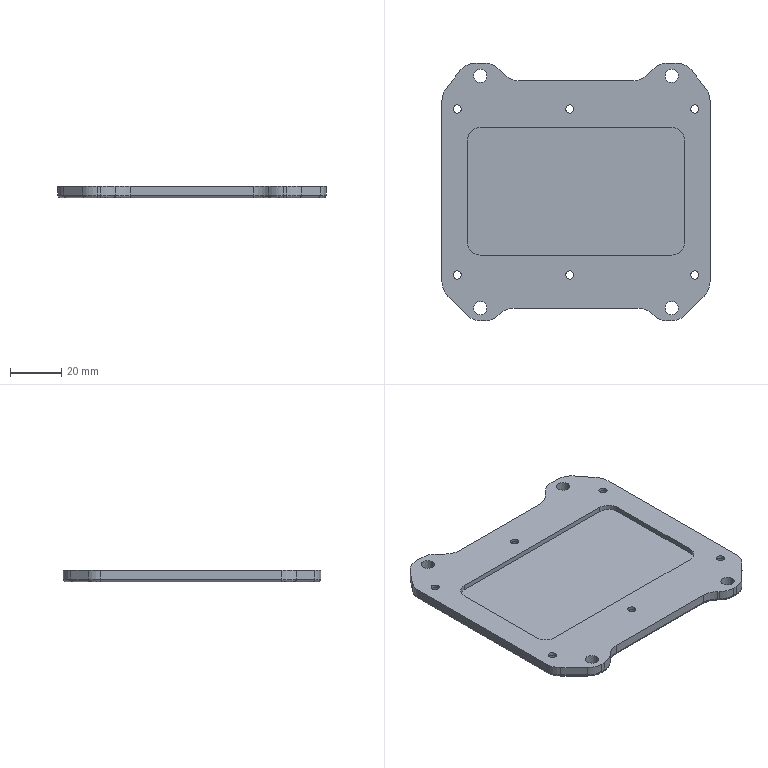NC program | NX | posted with a generic post | part box 105 x 101 x 4.5 mm
Lines 736 to 1574 of 30641:
(PLANAR_MILL_1 , TOOL : D4-12-D4-50-3T-FINISH)
N1452 T04 M6
N1454 G53
N1456 G17 G0 G90 X-47.229 Y-31.877 S4500 M3
N1458 G43 Z20. H4
N1460 Z0.5
N1462 G94 G1 X-47.45 Y-32.259 Z0.485 F500.
N1464 Y-32.741 Z0.468
N1466 X-47.183 Y-33.202 Z0.449
N1468 X-46.767 Y-33.443 Z0.432
N1470 X-46.251 Y-33.448 Z0.414
N1472 X-45.804 Y-33.19 Z0.396
N1474 X-45.55 Y-32.741 Z0.378
N1476 Y-32.259 Z0.362
N1478 X-45.804 Y-31.81 Z0.343
N1480 X-46.251 Y-31.552 Z0.325
N1482 X-46.767 Y-31.557 Z0.307
N1484 X-47.183 Y-31.798 Z0.291
N1486 X-47.45 Y-32.259 Z0.272
N1488 Y-32.741 Z0.255
N1490 X-47.183 Y-33.202 Z0.237
N1492 X-46.767 Y-33.443 Z0.22
N1494 X-46.251 Y-33.448 Z0.202
N1496 X-45.804 Y-33.19 Z0.184
N1498 X-45.55 Y-32.741 Z0.166
N1500 Y-32.259 Z0.149
N1502 X-45.804 Y-31.81 Z0.131
N1504 X-46.251 Y-31.552 Z0.113
N1506 X-46.767 Y-31.557 Z0.095
N1508 X-47.183 Y-31.798 Z0.078
N1510 X-47.45 Y-32.259 Z0.059
N1512 Y-32.741 Z0.043
N1514 X-47.183 Y-33.202 Z0.024
N1516 X-46.767 Y-33.443 Z0.007
N1518 X-46.251 Y-33.448 Z-0.011
N1520 X-45.804 Y-33.19 Z-0.029
N1522 X-45.55 Y-32.741 Z-0.047
N1524 Y-32.259 Z-0.064
N1526 X-45.804 Y-31.81 Z-0.082
N1528 X-46.251 Y-31.552 Z-0.1
N1530 X-46.767 Y-31.557 Z-0.118
N1532 X-47.183 Y-31.798 Z-0.134
N1534 X-47.45 Y-32.259 Z-0.153
N1536 Y-32.741 Z-0.17
N1538 X-47.183 Y-33.202 Z-0.189
N1540 X-46.767 Y-33.443 Z-0.205
N1542 X-46.251 Y-33.448 Z-0.223
N1544 X-45.804 Y-33.19 Z-0.241
N1546 X-45.55 Y-32.741 Z-0.259
N1548 Y-32.259 Z-0.276
N1550 X-45.804 Y-31.81 Z-0.294
N1552 X-46.251 Y-31.552 Z-0.312
N1554 X-46.767 Y-31.557 Z-0.33
N1556 X-47.183 Y-31.798 Z-0.347
N1558 X-47.45 Y-32.259 Z-0.366
N1560 Y-32.741 Z-0.382
N1562 X-47.183 Y-33.202 Z-0.401
N1564 X-46.767 Y-33.443 Z-0.418
N1566 X-46.251 Y-33.448 Z-0.436
N1568 X-45.804 Y-33.19 Z-0.454
N1570 X-45.55 Y-32.741 Z-0.472
N1572 Y-32.259 Z-0.489
N1574 X-45.804 Y-31.81 Z-0.507
N1576 X-46.251 Y-31.552 Z-0.525
N1578 X-46.767 Y-31.557 Z-0.543
N1580 X-47.183 Y-31.798 Z-0.56
N1582 X-47.45 Y-32.259 Z-0.578
N1584 Y-32.741 Z-0.595
N1586 X-47.183 Y-33.202 Z-0.614
N1588 X-46.767 Y-33.443 Z-0.63
N1590 X-46.251 Y-33.448 Z-0.648
N1592 X-45.804 Y-33.19 Z-0.667
N1594 X-45.55 Y-32.741 Z-0.685
N1596 Y-32.259 Z-0.701
N1598 X-45.804 Y-31.81 Z-0.719
N1600 X-46.251 Y-31.552 Z-0.737
N1602 X-46.767 Y-31.557 Z-0.755
N1604 X-47.183 Y-31.798 Z-0.772
N1606 X-47.45 Y-32.259 Z-0.791
N1608 Y-32.741 Z-0.808
N1610 X-47.183 Y-33.202 Z-0.826
N1612 X-46.767 Y-33.443 Z-0.843
N1614 X-46.251 Y-33.448 Z-0.861
N1616 X-45.804 Y-33.19 Z-0.879
N1618 X-45.55 Y-32.741 Z-0.897
N1620 Y-32.259 Z-0.914
N1622 X-45.804 Y-31.81 Z-0.932
N1624 X-46.251 Y-31.552 Z-0.95
N1626 X-46.767 Y-31.557 Z-0.968
N1628 X-47.183 Y-31.798 Z-0.985
N1630 X-47.45 Y-32.259 Z-1.003
N1632 Y-32.741 Z-1.02
N1634 X-47.183 Y-33.202 Z-1.039
N1636 X-46.767 Y-33.443 Z-1.056
N1638 X-46.251 Y-33.448 Z-1.074
N1640 X-45.804 Y-33.19 Z-1.092
N1642 X-45.55 Y-32.741 Z-1.11
N1644 Y-32.259 Z-1.126
N1646 X-45.804 Y-31.81 Z-1.144
N1648 X-46.251 Y-31.552 Z-1.162
N1650 X-46.767 Y-31.557 Z-1.181
N1652 X-47.183 Y-31.798 Z-1.197
N1654 X-47.45 Y-32.259 Z-1.216
N1656 Y-32.741 Z-1.233
N1658 X-47.183 Y-33.202 Z-1.251
N1660 X-46.767 Y-33.443 Z-1.268
N1662 X-46.251 Y-33.448 Z-1.286
N1664 X-45.804 Y-33.19 Z-1.304
N1666 X-45.55 Y-32.741 Z-1.322
N1668 Y-32.259 Z-1.339
N1670 X-45.804 Y-31.81 Z-1.357
N1672 X-46.251 Y-31.552 Z-1.375
N1674 X-46.767 Y-31.557 Z-1.393
N1676 X-47.183 Y-31.798 Z-1.41
N1678 X-47.45 Y-32.259 Z-1.429
N1680 Y-32.741 Z-1.445
N1682 X-47.183 Y-33.202 Z-1.464
N1684 X-46.767 Y-33.443 Z-1.481
N1686 X-46.251 Y-33.448 Z-1.499
N1688 X-45.804 Y-33.19 Z-1.517
N1690 X-45.55 Y-32.741 Z-1.535
N1692 Y-32.259 Z-1.552
N1694 X-45.804 Y-31.81 Z-1.57
N1696 X-46.251 Y-31.552 Z-1.588
N1698 X-46.767 Y-31.557 Z-1.606
N1700 X-47.183 Y-31.798 Z-1.622
N1702 X-47.45 Y-32.259 Z-1.641
N1704 Y-32.741 Z-1.658
N1706 X-47.183 Y-33.202 Z-1.676
N1708 X-46.767 Y-33.443 Z-1.693
N1710 X-46.251 Y-33.448 Z-1.711
N1712 X-45.804 Y-33.19 Z-1.729
N1714 X-45.55 Y-32.741 Z-1.747
N1716 Y-32.259 Z-1.764
N1718 X-45.804 Y-31.81 Z-1.782
N1720 X-46.251 Y-31.552 Z-1.8
N1722 X-46.767 Y-31.557 Z-1.818
N1724 X-47.183 Y-31.798 Z-1.835
N1726 X-47.45 Y-32.259 Z-1.854
N1728 Y-32.741 Z-1.87
N1730 X-47.183 Y-33.202 Z-1.889
N1732 X-46.767 Y-33.443 Z-1.906
N1734 X-46.251 Y-33.448 Z-1.924
N1736 X-45.804 Y-33.19 Z-1.942
N1738 X-45.55 Y-32.741 Z-1.96
N1740 Y-32.259 Z-1.977
N1742 X-45.804 Y-31.81 Z-1.995
N1744 X-46.251 Y-31.552 Z-2.013
N1746 X-46.767 Y-31.557 Z-2.031
N1748 X-47.183 Y-31.798 Z-2.048
N1750 X-47.45 Y-32.259 Z-2.066
N1752 Y-32.741 Z-2.083
N1754 X-47.183 Y-33.202 Z-2.102
N1756 X-46.767 Y-33.443 Z-2.118
N1758 X-46.251 Y-33.448 Z-2.136
N1760 X-45.804 Y-33.19 Z-2.154
N1762 X-45.55 Y-32.741 Z-2.172
N1764 Y-32.259 Z-2.189
N1766 X-45.804 Y-31.81 Z-2.207
N1768 X-46.251 Y-31.552 Z-2.225
N1770 X-46.767 Y-31.557 Z-2.243
N1772 X-47.183 Y-31.798 Z-2.26
N1774 X-47.45 Y-32.259 Z-2.279
N1776 Y-32.741 Z-2.296
N1778 X-47.183 Y-33.202 Z-2.314
N1780 X-46.767 Y-33.443 Z-2.331
N1782 X-46.251 Y-33.448 Z-2.349
N1784 X-45.804 Y-33.19 Z-2.367
N1786 X-45.55 Y-32.741 Z-2.385
N1788 Y-32.259 Z-2.402
N1790 X-45.804 Y-31.81 Z-2.42
N1792 X-46.251 Y-31.552 Z-2.438
N1794 X-46.767 Y-31.557 Z-2.456
N1796 X-47.183 Y-31.798 Z-2.473
N1798 X-47.45 Y-32.259 Z-2.491
N1800 Y-32.741 Z-2.508
N1802 X-47.183 Y-33.202 Z-2.527
N1804 X-46.767 Y-33.443 Z-2.544
N1806 X-46.251 Y-33.448 Z-2.562
N1808 X-45.804 Y-33.19 Z-2.58
N1810 X-45.55 Y-32.741 Z-2.598
N1812 Y-32.259 Z-2.614
N1814 X-45.804 Y-31.81 Z-2.632
N1816 X-46.251 Y-31.552 Z-2.65
N1818 X-46.767 Y-31.557 Z-2.668
N1820 X-47.183 Y-31.798 Z-2.685
N1822 X-47.45 Y-32.259 Z-2.704
N1824 Y-32.741 Z-2.721
N1826 X-47.183 Y-33.202 Z-2.739
N1828 X-46.767 Y-33.443 Z-2.756
N1830 X-46.251 Y-33.448 Z-2.774
N1832 X-45.804 Y-33.19 Z-2.792
N1834 X-45.55 Y-32.741 Z-2.81
N1836 Y-32.259 Z-2.827
N1838 X-45.804 Y-31.81 Z-2.845
N1840 X-46.251 Y-31.552 Z-2.863
N1842 X-46.767 Y-31.557 Z-2.881
N1844 X-47.183 Y-31.798 Z-2.898
N1846 X-47.45 Y-32.259 Z-2.916
N1848 Y-32.741 Z-2.933
N1850 X-47.183 Y-33.202 Z-2.952
N1852 X-46.767 Y-33.443 Z-2.969
N1854 X-46.251 Y-33.448 Z-2.987
N1856 X-45.804 Y-33.19 Z-3.005
N1858 X-45.55 Y-32.741 Z-3.023
N1860 Y-32.259 Z-3.04
N1862 X-45.804 Y-31.81 Z-3.058
N1864 X-46.251 Y-31.552 Z-3.076
N1866 X-46.767 Y-31.557 Z-3.094
N1868 X-47.183 Y-31.798 Z-3.11
N1870 X-47.45 Y-32.259 Z-3.129
N1872 Y-32.741 Z-3.146
N1874 X-47.183 Y-33.202 Z-3.164
N1876 X-46.767 Y-33.443 Z-3.181
N1878 X-46.251 Y-33.448 Z-3.199
N1880 X-45.804 Y-33.19 Z-3.217
N1882 X-45.55 Y-32.741 Z-3.235
N1884 Y-32.259 Z-3.252
N1886 X-45.804 Y-31.81 Z-3.27
N1888 X-46.251 Y-31.552 Z-3.288
N1890 X-46.767 Y-31.557 Z-3.306
N1892 X-47.183 Y-31.798 Z-3.323
N1894 X-47.45 Y-32.259 Z-3.342
N1896 Y-32.5 Z-3.35
N1898 G3 X-46.5 Y-33.45 R0.95
N1900 X-47.45 Y-32.5 R-0.95
N1902 G1 Z-2.85
N1904 G0 Z20.
N1906 X1.771 Y-31.877
N1908 Z0.5
N1910 G1 X1.55 Y-32.259 Z0.485
N1912 Y-32.741 Z0.468
N1914 X1.817 Y-33.202 Z0.449
N1916 X2.233 Y-33.443 Z0.432
N1918 X2.749 Y-33.448 Z0.414
N1920 X3.196 Y-33.19 Z0.396
N1922 X3.45 Y-32.741 Z0.378
N1924 Y-32.259 Z0.362
N1926 X3.196 Y-31.81 Z0.343
N1928 X2.749 Y-31.552 Z0.325
N1930 X2.233 Y-31.557 Z0.307
N1932 X1.817 Y-31.798 Z0.291
N1934 X1.55 Y-32.259 Z0.272
N1936 Y-32.741 Z0.255
N1938 X1.817 Y-33.202 Z0.237
N1940 X2.233 Y-33.443 Z0.22
N1942 X2.749 Y-33.448 Z0.202
N1944 X3.196 Y-33.19 Z0.184
N1946 X3.45 Y-32.741 Z0.166
N1948 Y-32.259 Z0.149
N1950 X3.196 Y-31.81 Z0.131
N1952 X2.749 Y-31.552 Z0.113
N1954 X2.233 Y-31.557 Z0.095
N1956 X1.817 Y-31.798 Z0.078
N1958 X1.55 Y-32.259 Z0.059
N1960 Y-32.741 Z0.043
N1962 X1.817 Y-33.202 Z0.024
N1964 X2.233 Y-33.443 Z0.007
N1966 X2.749 Y-33.448 Z-0.011
N1968 X3.196 Y-33.19 Z-0.029
N1970 X3.45 Y-32.741 Z-0.047
N1972 Y-32.259 Z-0.064
N1974 X3.196 Y-31.81 Z-0.082
N1976 X2.749 Y-31.552 Z-0.1
N1978 X2.233 Y-31.557 Z-0.118
N1980 X1.817 Y-31.798 Z-0.134
N1982 X1.55 Y-32.259 Z-0.153
N1984 Y-32.741 Z-0.17
N1986 X1.817 Y-33.202 Z-0.189
N1988 X2.233 Y-33.443 Z-0.205
N1990 X2.749 Y-33.448 Z-0.223
N1992 X3.196 Y-33.19 Z-0.241
N1994 X3.45 Y-32.741 Z-0.259
N1996 Y-32.259 Z-0.276
N1998 X3.196 Y-31.81 Z-0.294
N2000 X2.749 Y-31.552 Z-0.312
N2002 X2.233 Y-31.557 Z-0.33
N2004 X1.817 Y-31.798 Z-0.347
N2006 X1.55 Y-32.259 Z-0.366
N2008 Y-32.741 Z-0.382
N2010 X1.817 Y-33.202 Z-0.401
N2012 X2.233 Y-33.443 Z-0.418
N2014 X2.749 Y-33.448 Z-0.436
N2016 X3.196 Y-33.19 Z-0.454
N2018 X3.45 Y-32.741 Z-0.472
N2020 Y-32.259 Z-0.489
N2022 X3.196 Y-31.81 Z-0.507
N2024 X2.749 Y-31.552 Z-0.525
N2026 X2.233 Y-31.557 Z-0.543
N2028 X1.817 Y-31.798 Z-0.56
N2030 X1.55 Y-32.259 Z-0.578
N2032 Y-32.741 Z-0.595
N2034 X1.817 Y-33.202 Z-0.614
N2036 X2.233 Y-33.443 Z-0.63
N2038 X2.749 Y-33.448 Z-0.648
N2040 X3.196 Y-33.19 Z-0.667
N2042 X3.45 Y-32.741 Z-0.685
N2044 Y-32.259 Z-0.701
N2046 X3.196 Y-31.81 Z-0.719
N2048 X2.749 Y-31.552 Z-0.737
N2050 X2.233 Y-31.557 Z-0.755
N2052 X1.817 Y-31.798 Z-0.772
N2054 X1.55 Y-32.259 Z-0.791
N2056 Y-32.741 Z-0.808
N2058 X1.817 Y-33.202 Z-0.826
N2060 X2.233 Y-33.443 Z-0.843
N2062 X2.749 Y-33.448 Z-0.861
N2064 X3.196 Y-33.19 Z-0.879
N2066 X3.45 Y-32.741 Z-0.897
N2068 Y-32.259 Z-0.914
N2070 X3.196 Y-31.81 Z-0.932
N2072 X2.749 Y-31.552 Z-0.95
N2074 X2.233 Y-31.557 Z-0.968
N2076 X1.817 Y-31.798 Z-0.985
N2078 X1.55 Y-32.259 Z-1.003
N2080 Y-32.741 Z-1.02
N2082 X1.817 Y-33.202 Z-1.039
N2084 X2.233 Y-33.443 Z-1.056
N2086 X2.749 Y-33.448 Z-1.074
N2088 X3.196 Y-33.19 Z-1.092
N2090 X3.45 Y-32.741 Z-1.11
N2092 Y-32.259 Z-1.126
N2094 X3.196 Y-31.81 Z-1.144
N2096 X2.749 Y-31.552 Z-1.162
N2098 X2.233 Y-31.557 Z-1.181
N2100 X1.817 Y-31.798 Z-1.197
N2102 X1.55 Y-32.259 Z-1.216
N2104 Y-32.741 Z-1.233
N2106 X1.817 Y-33.202 Z-1.251
N2108 X2.233 Y-33.443 Z-1.268
N2110 X2.749 Y-33.448 Z-1.286
N2112 X3.196 Y-33.19 Z-1.304
N2114 X3.45 Y-32.741 Z-1.322
N2116 Y-32.259 Z-1.339
N2118 X3.196 Y-31.81 Z-1.357
N2120 X2.749 Y-31.552 Z-1.375
N2122 X2.233 Y-31.557 Z-1.393
N2124 X1.817 Y-31.798 Z-1.41
N2126 X1.55 Y-32.259 Z-1.429
N2128 Y-32.741 Z-1.445
N2130 X1.817 Y-33.202 Z-1.464
N2132 X2.233 Y-33.443 Z-1.481
N2134 X2.749 Y-33.448 Z-1.499
N2136 X3.196 Y-33.19 Z-1.517
N2138 X3.45 Y-32.741 Z-1.535
N2140 Y-32.259 Z-1.552
N2142 X3.196 Y-31.81 Z-1.57
N2144 X2.749 Y-31.552 Z-1.588
N2146 X2.233 Y-31.557 Z-1.606
N2148 X1.817 Y-31.798 Z-1.622
N2150 X1.55 Y-32.259 Z-1.641
N2152 Y-32.741 Z-1.658
N2154 X1.817 Y-33.202 Z-1.676
N2156 X2.233 Y-33.443 Z-1.693
N2158 X2.749 Y-33.448 Z-1.711
N2160 X3.196 Y-33.19 Z-1.729
N2162 X3.45 Y-32.741 Z-1.747
N2164 Y-32.259 Z-1.764
N2166 X3.196 Y-31.81 Z-1.782
N2168 X2.749 Y-31.552 Z-1.8
N2170 X2.233 Y-31.557 Z-1.818
N2172 X1.817 Y-31.798 Z-1.835
N2174 X1.55 Y-32.259 Z-1.854
N2176 Y-32.741 Z-1.87
N2178 X1.817 Y-33.202 Z-1.889
N2180 X2.233 Y-33.443 Z-1.906
N2182 X2.749 Y-33.448 Z-1.924
N2184 X3.196 Y-33.19 Z-1.942
N2186 X3.45 Y-32.741 Z-1.96
N2188 Y-32.259 Z-1.977
N2190 X3.196 Y-31.81 Z-1.995
N2192 X2.749 Y-31.552 Z-2.013
N2194 X2.233 Y-31.557 Z-2.031
N2196 X1.817 Y-31.798 Z-2.048
N2198 X1.55 Y-32.259 Z-2.066
N2200 Y-32.741 Z-2.083
N2202 X1.817 Y-33.202 Z-2.102
N2204 X2.233 Y-33.443 Z-2.118
N2206 X2.749 Y-33.448 Z-2.136
N2208 X3.196 Y-33.19 Z-2.154
N2210 X3.45 Y-32.741 Z-2.172
N2212 Y-32.259 Z-2.189
N2214 X3.196 Y-31.81 Z-2.207
N2216 X2.749 Y-31.552 Z-2.225
N2218 X2.233 Y-31.557 Z-2.243
N2220 X1.817 Y-31.798 Z-2.26
N2222 X1.55 Y-32.259 Z-2.279
N2224 Y-32.741 Z-2.296
N2226 X1.817 Y-33.202 Z-2.314
N2228 X2.233 Y-33.443 Z-2.331
N2230 X2.749 Y-33.448 Z-2.349
N2232 X3.196 Y-33.19 Z-2.367
N2234 X3.45 Y-32.741 Z-2.385
N2236 Y-32.259 Z-2.402
N2238 X3.196 Y-31.81 Z-2.42
N2240 X2.749 Y-31.552 Z-2.438
N2242 X2.233 Y-31.557 Z-2.456
N2244 X1.817 Y-31.798 Z-2.473
N2246 X1.55 Y-32.259 Z-2.491
N2248 Y-32.741 Z-2.508
N2250 X1.817 Y-33.202 Z-2.527
N2252 X2.233 Y-33.443 Z-2.544
N2254 X2.749 Y-33.448 Z-2.562
N2256 X3.196 Y-33.19 Z-2.58
N2258 X3.45 Y-32.741 Z-2.598
N2260 Y-32.259 Z-2.614
N2262 X3.196 Y-31.81 Z-2.632
N2264 X2.749 Y-31.552 Z-2.65
N2266 X2.233 Y-31.557 Z-2.668
N2268 X1.817 Y-31.798 Z-2.685
N2270 X1.55 Y-32.259 Z-2.704
N2272 Y-32.741 Z-2.721
N2274 X1.817 Y-33.202 Z-2.739
N2276 X2.233 Y-33.443 Z-2.756
N2278 X2.749 Y-33.448 Z-2.774
N2280 X3.196 Y-33.19 Z-2.792
N2282 X3.45 Y-32.741 Z-2.81
N2284 Y-32.259 Z-2.827
N2286 X3.196 Y-31.81 Z-2.845
N2288 X2.749 Y-31.552 Z-2.863
N2290 X2.233 Y-31.557 Z-2.881
N2292 X1.817 Y-31.798 Z-2.898
N2294 X1.55 Y-32.259 Z-2.916
N2296 Y-32.741 Z-2.933
N2298 X1.817 Y-33.202 Z-2.952
N2300 X2.233 Y-33.443 Z-2.969
N2302 X2.749 Y-33.448 Z-2.987
N2304 X3.196 Y-33.19 Z-3.005
N2306 X3.45 Y-32.741 Z-3.023
N2308 Y-32.259 Z-3.04
N2310 X3.196 Y-31.81 Z-3.058
N2312 X2.749 Y-31.552 Z-3.076
N2314 X2.233 Y-31.557 Z-3.094
N2316 X1.817 Y-31.798 Z-3.11
N2318 X1.55 Y-32.259 Z-3.129
N2320 Y-32.741 Z-3.146
N2322 X1.817 Y-33.202 Z-3.164
N2324 X2.233 Y-33.443 Z-3.181
N2326 X2.749 Y-33.448 Z-3.199
N2328 X3.196 Y-33.19 Z-3.217
N2330 X3.45 Y-32.741 Z-3.235
N2332 Y-32.259 Z-3.252
N2334 X3.196 Y-31.81 Z-3.27
N2336 X2.749 Y-31.552 Z-3.288
N2338 X2.233 Y-31.557 Z-3.306
N2340 X1.817 Y-31.798 Z-3.323
N2342 X1.55 Y-32.259 Z-3.342
N2344 Y-32.5 Z-3.35
N2346 G3 X2.5 Y-33.45 R0.95
N2348 X1.55 Y-32.5 R-0.95
N2350 G1 Z-2.85
N2352 G0 Z20.
N2354 X45.771 Y-31.877
N2356 Z0.5
N2358 G1 X45.55 Y-32.259 Z0.485
N2360 Y-32.741 Z0.468
N2362 X45.817 Y-33.202 Z0.449
N2364 X46.233 Y-33.443 Z0.432
N2366 X46.749 Y-33.448 Z0.414
N2368 X47.196 Y-33.19 Z0.396
N2370 X47.45 Y-32.741 Z0.378
N2372 Y-32.259 Z0.362
N2374 X47.196 Y-31.81 Z0.343
N2376 X46.749 Y-31.552 Z0.325
N2378 X46.233 Y-31.557 Z0.307
N2380 X45.817 Y-31.798 Z0.291
N2382 X45.55 Y-32.259 Z0.272
N2384 Y-32.741 Z0.255
N2386 X45.817 Y-33.202 Z0.237
N2388 X46.233 Y-33.443 Z0.22
N2390 X46.749 Y-33.448 Z0.202
N2392 X47.196 Y-33.19 Z0.184
N2394 X47.45 Y-32.741 Z0.166
N2396 Y-32.259 Z0.149
N2398 X47.196 Y-31.81 Z0.131
N2400 X46.749 Y-31.552 Z0.113
N2402 X46.233 Y-31.557 Z0.095
N2404 X45.817 Y-31.798 Z0.078
N2406 X45.55 Y-32.259 Z0.059
N2408 Y-32.741 Z0.043
N2410 X45.817 Y-33.202 Z0.024
N2412 X46.233 Y-33.443 Z0.007
N2414 X46.749 Y-33.448 Z-0.011
N2416 X47.196 Y-33.19 Z-0.029
N2418 X47.45 Y-32.741 Z-0.047
N2420 Y-32.259 Z-0.064
N2422 X47.196 Y-31.81 Z-0.082
N2424 X46.749 Y-31.552 Z-0.1
N2426 X46.233 Y-31.557 Z-0.118
N2428 X45.817 Y-31.798 Z-0.134
N2430 X45.55 Y-32.259 Z-0.153
N2432 Y-32.741 Z-0.17
N2434 X45.817 Y-33.202 Z-0.189
N2436 X46.233 Y-33.443 Z-0.205
N2438 X46.749 Y-33.448 Z-0.223
N2440 X47.196 Y-33.19 Z-0.241
N2442 X47.45 Y-32.741 Z-0.259
N2444 Y-32.259 Z-0.276
N2446 X47.196 Y-31.81 Z-0.294
N2448 X46.749 Y-31.552 Z-0.312
N2450 X46.233 Y-31.557 Z-0.33
N2452 X45.817 Y-31.798 Z-0.347
N2454 X45.55 Y-32.259 Z-0.366
N2456 Y-32.741 Z-0.382
N2458 X45.817 Y-33.202 Z-0.401
N2460 X46.233 Y-33.443 Z-0.418
N2462 X46.749 Y-33.448 Z-0.436
N2464 X47.196 Y-33.19 Z-0.454
N2466 X47.45 Y-32.741 Z-0.472
N2468 Y-32.259 Z-0.489
N2470 X47.196 Y-31.81 Z-0.507
N2472 X46.749 Y-31.552 Z-0.525
N2474 X46.233 Y-31.557 Z-0.543
N2476 X45.817 Y-31.798 Z-0.56
N2478 X45.55 Y-32.259 Z-0.578
N2480 Y-32.741 Z-0.595
N2482 X45.817 Y-33.202 Z-0.614
N2484 X46.233 Y-33.443 Z-0.63
N2486 X46.749 Y-33.448 Z-0.648
N2488 X47.196 Y-33.19 Z-0.667
N2490 X47.45 Y-32.741 Z-0.685
N2492 Y-32.259 Z-0.701
N2494 X47.196 Y-31.81 Z-0.719
N2496 X46.749 Y-31.552 Z-0.737
N2498 X46.233 Y-31.557 Z-0.755
N2500 X45.817 Y-31.798 Z-0.772
N2502 X45.55 Y-32.259 Z-0.791
N2504 Y-32.741 Z-0.808
N2506 X45.817 Y-33.202 Z-0.826
N2508 X46.233 Y-33.443 Z-0.843
N2510 X46.749 Y-33.448 Z-0.861
N2512 X47.196 Y-33.19 Z-0.879
N2514 X47.45 Y-32.741 Z-0.897
N2516 Y-32.259 Z-0.914
N2518 X47.196 Y-31.81 Z-0.932
N2520 X46.749 Y-31.552 Z-0.95
N2522 X46.233 Y-31.557 Z-0.968
N2524 X45.817 Y-31.798 Z-0.985
N2526 X45.55 Y-32.259 Z-1.003
N2528 Y-32.741 Z-1.02
N2530 X45.817 Y-33.202 Z-1.039
N2532 X46.233 Y-33.443 Z-1.056
N2534 X46.749 Y-33.448 Z-1.074
N2536 X47.196 Y-33.19 Z-1.092
N2538 X47.45 Y-32.741 Z-1.11
N2540 Y-32.259 Z-1.126
N2542 X47.196 Y-31.81 Z-1.144
N2544 X46.749 Y-31.552 Z-1.162
N2546 X46.233 Y-31.557 Z-1.181
N2548 X45.817 Y-31.798 Z-1.197
N2550 X45.55 Y-32.259 Z-1.216
N2552 Y-32.741 Z-1.233
N2554 X45.817 Y-33.202 Z-1.251
N2556 X46.233 Y-33.443 Z-1.268
N2558 X46.749 Y-33.448 Z-1.286
N2560 X47.196 Y-33.19 Z-1.304
N2562 X47.45 Y-32.741 Z-1.322
N2564 Y-32.259 Z-1.339
N2566 X47.196 Y-31.81 Z-1.357
N2568 X46.749 Y-31.552 Z-1.375
N2570 X46.233 Y-31.557 Z-1.393
N2572 X45.817 Y-31.798 Z-1.41
N2574 X45.55 Y-32.259 Z-1.429
N2576 Y-32.741 Z-1.445
N2578 X45.817 Y-33.202 Z-1.464
N2580 X46.233 Y-33.443 Z-1.481
N2582 X46.749 Y-33.448 Z-1.499
N2584 X47.196 Y-33.19 Z-1.517
N2586 X47.45 Y-32.741 Z-1.535
N2588 Y-32.259 Z-1.552
N2590 X47.196 Y-31.81 Z-1.57
N2592 X46.749 Y-31.552 Z-1.588
N2594 X46.233 Y-31.557 Z-1.606
N2596 X45.817 Y-31.798 Z-1.622
N2598 X45.55 Y-32.259 Z-1.641
N2600 Y-32.741 Z-1.658
N2602 X45.817 Y-33.202 Z-1.676
N2604 X46.233 Y-33.443 Z-1.693
N2606 X46.749 Y-33.448 Z-1.711
N2608 X47.196 Y-33.19 Z-1.729
N2610 X47.45 Y-32.741 Z-1.747
N2612 Y-32.259 Z-1.764
N2614 X47.196 Y-31.81 Z-1.782
N2616 X46.749 Y-31.552 Z-1.8
N2618 X46.233 Y-31.557 Z-1.818
N2620 X45.817 Y-31.798 Z-1.835
N2622 X45.55 Y-32.259 Z-1.854
N2624 Y-32.741 Z-1.87
N2626 X45.817 Y-33.202 Z-1.889
N2628 X46.233 Y-33.443 Z-1.906
N2630 X46.749 Y-33.448 Z-1.924
N2632 X47.196 Y-33.19 Z-1.942
N2634 X47.45 Y-32.741 Z-1.96
N2636 Y-32.259 Z-1.977
N2638 X47.196 Y-31.81 Z-1.995
N2640 X46.749 Y-31.552 Z-2.013
N2642 X46.233 Y-31.557 Z-2.031
N2644 X45.817 Y-31.798 Z-2.048
N2646 X45.55 Y-32.259 Z-2.066
N2648 Y-32.741 Z-2.083
N2650 X45.817 Y-33.202 Z-2.102
N2652 X46.233 Y-33.443 Z-2.118
N2654 X46.749 Y-33.448 Z-2.136
N2656 X47.196 Y-33.19 Z-2.154
N2658 X47.45 Y-32.741 Z-2.172
N2660 Y-32.259 Z-2.189
N2662 X47.196 Y-31.81 Z-2.207
N2664 X46.749 Y-31.552 Z-2.225
N2666 X46.233 Y-31.557 Z-2.243
N2668 X45.817 Y-31.798 Z-2.26
N2670 X45.55 Y-32.259 Z-2.279
N2672 Y-32.741 Z-2.296
N2674 X45.817 Y-33.202 Z-2.314
N2676 X46.233 Y-33.443 Z-2.331
N2678 X46.749 Y-33.448 Z-2.349
N2680 X47.196 Y-33.19 Z-2.367
N2682 X47.45 Y-32.741 Z-2.385
N2684 Y-32.259 Z-2.402
N2686 X47.196 Y-31.81 Z-2.42
N2688 X46.749 Y-31.552 Z-2.438
N2690 X46.233 Y-31.557 Z-2.456
N2692 X45.817 Y-31.798 Z-2.473
N2694 X45.55 Y-32.259 Z-2.491
N2696 Y-32.741 Z-2.508
N2698 X45.817 Y-33.202 Z-2.527
N2700 X46.233 Y-33.443 Z-2.544
N2702 X46.749 Y-33.448 Z-2.562
N2704 X47.196 Y-33.19 Z-2.58
N2706 X47.45 Y-32.741 Z-2.598
N2708 Y-32.259 Z-2.614
N2710 X47.196 Y-31.81 Z-2.632
N2712 X46.749 Y-31.552 Z-2.65
N2714 X46.233 Y-31.557 Z-2.668
N2716 X45.817 Y-31.798 Z-2.685
N2718 X45.55 Y-32.259 Z-2.704
N2720 Y-32.741 Z-2.721
N2722 X45.817 Y-33.202 Z-2.739
N2724 X46.233 Y-33.443 Z-2.756
N2726 X46.749 Y-33.448 Z-2.774
N2728 X47.196 Y-33.19 Z-2.792
N2730 X47.45 Y-32.741 Z-2.81
N2732 Y-32.259 Z-2.827
N2734 X47.196 Y-31.81 Z-2.845
N2736 X46.749 Y-31.552 Z-2.863
N2738 X46.233 Y-31.557 Z-2.881
N2740 X45.817 Y-31.798 Z-2.898
N2742 X45.55 Y-32.259 Z-2.916
N2744 Y-32.741 Z-2.933
N2746 X45.817 Y-33.202 Z-2.952
N2748 X46.233 Y-33.443 Z-2.969
N2750 X46.749 Y-33.448 Z-2.987
N2752 X47.196 Y-33.19 Z-3.005
N2754 X47.45 Y-32.741 Z-3.023
N2756 Y-32.259 Z-3.04
N2758 X47.196 Y-31.81 Z-3.058
N2760 X46.749 Y-31.552 Z-3.076
N2762 X46.233 Y-31.557 Z-3.094
N2764 X45.817 Y-31.798 Z-3.11
N2766 X45.55 Y-32.259 Z-3.129
N2768 Y-32.741 Z-3.146
N2770 X45.817 Y-33.202 Z-3.164
N2772 X46.233 Y-33.443 Z-3.181
N2774 X46.749 Y-33.448 Z-3.199
N2776 X47.196 Y-33.19 Z-3.217
N2778 X47.45 Y-32.741 Z-3.235
N2780 Y-32.259 Z-3.252
N2782 X47.196 Y-31.81 Z-3.27
N2784 X46.749 Y-31.552 Z-3.288
N2786 X46.233 Y-31.557 Z-3.306
N2788 X45.817 Y-31.798 Z-3.323
N2790 X45.55 Y-32.259 Z-3.342
N2792 Y-32.5 Z-3.35
N2794 G3 X46.5 Y-33.45 R0.95
N2796 X45.55 Y-32.5 R-0.95
N2798 G1 Z-2.85
N2800 G0 Z20.
N2802 X45.771 Y33.123
N2804 Z0.5
N2806 G1 X45.55 Y32.741 Z0.485
N2808 Y32.259 Z0.468
N2810 X45.817 Y31.798 Z0.449
N2812 X46.233 Y31.557 Z0.432
N2814 X46.749 Y31.552 Z0.414
N2816 X47.196 Y31.81 Z0.396
N2818 X47.45 Y32.259 Z0.378
N2820 Y32.741 Z0.362
N2822 X47.196 Y33.19 Z0.343
N2824 X46.749 Y33.448 Z0.325
N2826 X46.233 Y33.443 Z0.307
N2828 X45.817 Y33.202 Z0.291
N2830 X45.55 Y32.741 Z0.272
N2832 Y32.259 Z0.255
N2834 X45.817 Y31.798 Z0.237
N2836 X46.233 Y31.557 Z0.22
N2838 X46.749 Y31.552 Z0.202
N2840 X47.196 Y31.81 Z0.184
N2842 X47.45 Y32.259 Z0.166
N2844 Y32.741 Z0.149
N2846 X47.196 Y33.19 Z0.131
N2848 X46.749 Y33.448 Z0.113
N2850 X46.233 Y33.443 Z0.095
N2852 X45.817 Y33.202 Z0.078
N2854 X45.55 Y32.741 Z0.059
N2856 Y32.259 Z0.043
N2858 X45.817 Y31.798 Z0.024
N2860 X46.233 Y31.557 Z0.007
N2862 X46.749 Y31.552 Z-0.011
N2864 X47.196 Y31.81 Z-0.029
N2866 X47.45 Y32.259 Z-0.047
N2868 Y32.741 Z-0.064
N2870 X47.196 Y33.19 Z-0.082
N2872 X46.749 Y33.448 Z-0.1
N2874 X46.233 Y33.443 Z-0.118
N2876 X45.817 Y33.202 Z-0.134
N2878 X45.55 Y32.741 Z-0.153
N2880 Y32.259 Z-0.17
N2882 X45.817 Y31.798 Z-0.189
N2884 X46.233 Y31.557 Z-0.205
N2886 X46.749 Y31.552 Z-0.223
N2888 X47.196 Y31.81 Z-0.241
N2890 X47.45 Y32.259 Z-0.259
N2892 Y32.741 Z-0.276
N2894 X47.196 Y33.19 Z-0.294
N2896 X46.749 Y33.448 Z-0.312
N2898 X46.233 Y33.443 Z-0.33
N2900 X45.817 Y33.202 Z-0.347
N2902 X45.55 Y32.741 Z-0.366
N2904 Y32.259 Z-0.382
N2906 X45.817 Y31.798 Z-0.401
N2908 X46.233 Y31.557 Z-0.418
N2910 X46.749 Y31.552 Z-0.436
N2912 X47.196 Y31.81 Z-0.454
N2914 X47.45 Y32.259 Z-0.472
N2916 Y32.741 Z-0.489
N2918 X47.196 Y33.19 Z-0.507
N2920 X46.749 Y33.448 Z-0.525
N2922 X46.233 Y33.443 Z-0.543
N2924 X45.817 Y33.202 Z-0.56
N2926 X45.55 Y32.741 Z-0.578
N2928 Y32.259 Z-0.595
N2930 X45.817 Y31.798 Z-0.614
N2932 X46.233 Y31.557 Z-0.63
N2934 X46.749 Y31.552 Z-0.648
N2936 X47.196 Y31.81 Z-0.667
N2938 X47.45 Y32.259 Z-0.685
N2940 Y32.741 Z-0.701
N2942 X47.196 Y33.19 Z-0.719
N2944 X46.749 Y33.448 Z-0.737
N2946 X46.233 Y33.443 Z-0.755
N2948 X45.817 Y33.202 Z-0.772
N2950 X45.55 Y32.741 Z-0.791
N2952 Y32.259 Z-0.808
N2954 X45.817 Y31.798 Z-0.826
N2956 X46.233 Y31.557 Z-0.843
N2958 X46.749 Y31.552 Z-0.861
N2960 X47.196 Y31.81 Z-0.879
N2962 X47.45 Y32.259 Z-0.897
N2964 Y32.741 Z-0.914
N2966 X47.196 Y33.19 Z-0.932
N2968 X46.749 Y33.448 Z-0.95
N2970 X46.233 Y33.443 Z-0.968
N2972 X45.817 Y33.202 Z-0.985
N2974 X45.55 Y32.741 Z-1.003
N2976 Y32.259 Z-1.02
N2978 X45.817 Y31.798 Z-1.039
N2980 X46.233 Y31.557 Z-1.056
N2982 X46.749 Y31.552 Z-1.074
N2984 X47.196 Y31.81 Z-1.092
N2986 X47.45 Y32.259 Z-1.11
N2988 Y32.741 Z-1.126
N2990 X47.196 Y33.19 Z-1.144
N2992 X46.749 Y33.448 Z-1.162
N2994 X46.233 Y33.443 Z-1.181
N2996 X45.817 Y33.202 Z-1.197
N2998 X45.55 Y32.741 Z-1.216
N3000 Y32.259 Z-1.233
N3002 X45.817 Y31.798 Z-1.251
N3004 X46.233 Y31.557 Z-1.268
N3006 X46.749 Y31.552 Z-1.286
N3008 X47.196 Y31.81 Z-1.304
N3010 X47.45 Y32.259 Z-1.322
N3012 Y32.741 Z-1.339
N3014 X47.196 Y33.19 Z-1.357
N3016 X46.749 Y33.448 Z-1.375
N3018 X46.233 Y33.443 Z-1.393
N3020 X45.817 Y33.202 Z-1.41
N3022 X45.55 Y32.741 Z-1.429
N3024 Y32.259 Z-1.445
N3026 X45.817 Y31.798 Z-1.464
N3028 X46.233 Y31.557 Z-1.481
N3030 X46.749 Y31.552 Z-1.499
N3032 X47.196 Y31.81 Z-1.517
N3034 X47.45 Y32.259 Z-1.535
N3036 Y32.741 Z-1.552
N3038 X47.196 Y33.19 Z-1.57
N3040 X46.749 Y33.448 Z-1.588
N3042 X46.233 Y33.443 Z-1.606
N3044 X45.817 Y33.202 Z-1.622
N3046 X45.55 Y32.741 Z-1.641
N3048 Y32.259 Z-1.658
N3050 X45.817 Y31.798 Z-1.676
N3052 X46.233 Y31.557 Z-1.693
N3054 X46.749 Y31.552 Z-1.711
N3056 X47.196 Y31.81 Z-1.729
N3058 X47.45 Y32.259 Z-1.747
N3060 Y32.741 Z-1.764
N3062 X47.196 Y33.19 Z-1.782
N3064 X46.749 Y33.448 Z-1.8
N3066 X46.233 Y33.443 Z-1.818
N3068 X45.817 Y33.202 Z-1.835
N3070 X45.55 Y32.741 Z-1.854
N3072 Y32.259 Z-1.87
N3074 X45.817 Y31.798 Z-1.889
N3076 X46.233 Y31.557 Z-1.906
N3078 X46.749 Y31.552 Z-1.924
N3080 X47.196 Y31.81 Z-1.942
N3082 X47.45 Y32.259 Z-1.96
N3084 Y32.741 Z-1.977
N3086 X47.196 Y33.19 Z-1.995
N3088 X46.749 Y33.448 Z-2.013
N3090 X46.233 Y33.443 Z-2.031
N3092 X45.817 Y33.202 Z-2.048
N3094 X45.55 Y32.741 Z-2.066
N3096 Y32.259 Z-2.083
N3098 X45.817 Y31.798 Z-2.102
N3100 X46.233 Y31.557 Z-2.118
N3102 X46.749 Y31.552 Z-2.136
N3104 X47.196 Y31.81 Z-2.154
N3106 X47.45 Y32.259 Z-2.172
N3108 Y32.741 Z-2.189
N3110 X47.196 Y33.19 Z-2.207
N3112 X46.749 Y33.448 Z-2.225
N3114 X46.233 Y33.443 Z-2.243
N3116 X45.817 Y33.202 Z-2.26
N3118 X45.55 Y32.741 Z-2.279
N3120 Y32.259 Z-2.296
N3122 X45.817 Y31.798 Z-2.314